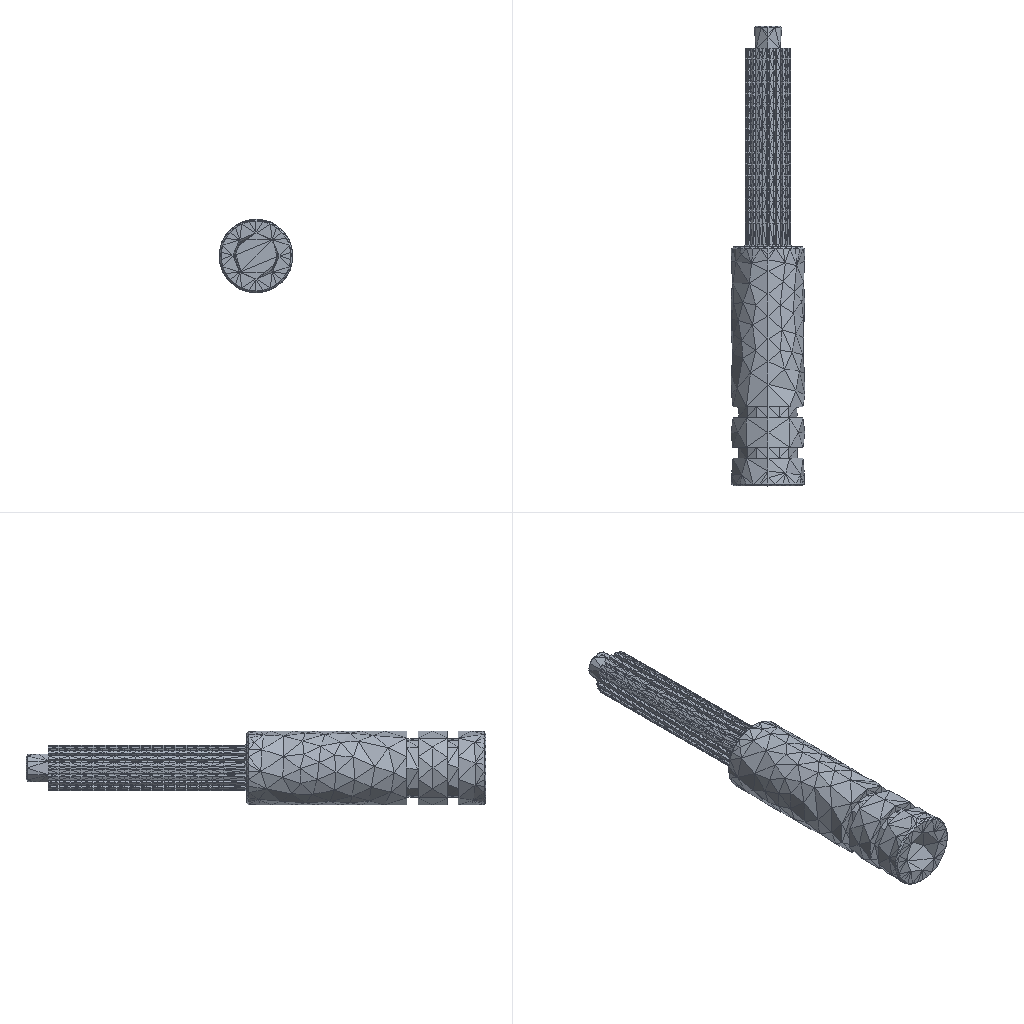Simulation study | ansys workbench
Ansys APDL input file, long lists of numbers shortened:
/batch
/config,noeldb,1     ! force off writing results to database
*get,_wallstrt,active,,time,wall
! ANSYS input file written by Workbench version 2022 R1
! File used for geometry attach: F:\ansys（分析文件汇总)\ansys转向器有限元分析\转向器\分析\齿条.STEP
/title,wbnew--____ (E5)
! ****** Begin Custom Load Command Snippet ******
/COM, ACT Extensions:
/COM,     LSDYNA, 2021.1
/COM,
! ****** End   Custom Load Command Snippet ******
*DIM,_wb_ProjectScratch_dir,string,248
_wb_ProjectScratch_dir(1) = 'C:\Users\Administrator\AppData\Local\Temp\WB_Administrator_18756_2\_ProjectScratch\Scr7D70\'
*DIM,_wb_SolverFiles_dir,string,248
_wb_SolverFiles_dir(1) = 'C:\Users\Administrator\AppData\Local\Temp\WB_Administrator_18756_2\wbnew_files\dp0\SYS-1\MECH\'
*DIM,_wb_userfiles_dir,string,248
_wb_userfiles_dir(1) = 'C:\Users\Administrator\AppData\Local\Temp\WB_Administrator_18756_2\wbnew_files\user_files\'
/com,--- Data in consistent NMM units. See Solving Units in the help system for more information.
/units,MPA
/nopr
/wb,file,start              !  signify a WB generated input file
/prep7
! Turn off shape checking because checks already performed inside WB mesher.
! See help system for more information.
SHPP,OFF,,NOWARN
/nolist
etcon,set             ! allow ANSYS to choose best KEYOP's for 180x elements, resets any applicable keyopt to MAPDL defaults
/com,*********** Nodes for the whole assembly ***********
nblock,3,,8393
(1i9,3e20.9e3)
        1    -9.866055935E-15    -3.500000000E+01     4.985000000E+02
! (7629 more lines like these left out)
-1
/wb,elem,start            !  set before creation of elements
/com,*********** Elements for Body 1 "__-FreeParts|__-__4" ***********
et,1,187
eblock,19,solid,,3600
(19i9)
        1        1        1        1        0        0        0        0       10        0        1      682     1334     1374     1348     5617     7596     5619     5618
! (7199 more lines like these left out)
-1
/wb,elem,end               !  done creating elements
/com,*********** Send User Defined Coordinate System(s) ***********
csys,0
toffst,273.15,  ! Temperature offset from absolute zero
/com,*********** Set Reference Temperature ***********
tref,22.
/wb,mat,start              !  starting to send materials
/com,*********** Send Materials ***********
Temperature = 'TEMP' ! Temperature
MP,DENS,1,7.85e-09,	! tonne mm^-3
MP,ALPX,1,1.2e-05,	! C^-1
MP,C,1,434000000,	! mm^2 s^-2 C^-1
MP,KXX,1,60.5,	! tonne mm s^-3 C^-1
MP,RSVX,1,0.00017,	! ohm mm
MP,EX,1,200000,	! tonne s^-2 mm^-1
MP,NUXY,1,0.3,
MP,MURX,1,10000,
/wb,mat,end                !  done sending materials
!************************* Model Summary ********************
!__-FreeParts|__-__4,	结构钢,	matid,	1
!************************* End Model Summary ********************
! get the diagonal of the bounding box. Needed later for other things
*get,_xmin,node,,mnloc,x
*get,_ymin,node,,mnloc,y
*get,_zmin,node,,mnloc,z
*get,_xmax,node,,mxloc,x
*get,_ymax,node,,mxloc,y
*get,_zmax,node,,mxloc,z
_ASMDIAG=(_xmax-_xmin)*(_xmax-_xmin)+(_ymax-_ymin)*(_ymax-_ymin)+(_zmax-_zmin)*(_zmax-_zmin)
_ASMDIAG=SQRT(_ASMDIAG)
/wb,contact,start          !  starting to send contact
/wb,contact,end            !  done creating contacts
/com,*********** Send Named Selection as Node Component ***********
CMBLOCK,______  ,NODE,      744
(8i10)
       207       208       211       212       215       216       219       220
! (92 more lines like these left out)
/golist
/wb,load,start             !  starting to send loads
/com,*********** Fixed Supports ***********
CMBLOCK,_FIXEDSU,NODE,      343
(8i10)
        21        22        23        24        25        36        37        38
! (42 more lines like these left out)
cmsel,s,_FIXEDSU
d,all,all
nsel,all
/com,*********** Define Force Using Surface Effect Elements ***********
local,12,0,0.,0.,0.,0.,0.,0.
csys,0
et,2,154
eblock,10,,,198
(15i9)
     6139        2        2        2       12      413      450      942      942     4067     4272      942     4072
! (197 more lines like these left out)
-1
esel,s,type,,2
keyop,2,2,1                ! Apply load in local coordinate system
keyop,2,7,1                ! Use original area so load is constant in large deformation
esel,all
/gst,on,on
fini
*get,_numnode,node,0,count
*get,_numelem,elem,0,count
*get, _MAXELEMNUM, elem, 0, NUM, MAX
*get, _MAXNODENUM, node, 0, NUM, MAX
*get, _MAXELEMTYPE, etyp, 0, NUM, MAX
*get, _MAXREALCONST, real, 0, NUM, MAX
/go
/wb,load,end               !  done creating loads
/com,--- Number of total nodes = %_numnode%
/com,--- Number of contact elements = 198
/com,--- Number of spring elements = 0
/com,--- Number of bearing elements = 0
/com,--- Number of solid elements = 3600
/com,--- Number of condensed parts = 0
/com,--- Number of total elements = %_numelem%
*get,_wallbsol,active,,time,wall
/com,****************************************************************************
/com,*************************    SOLUTION       ********************************
/com,****************************************************************************
/solu
antype,0                   ! static analysis
_thickRatio=  0     ! Ratio of thick parts in the model
eqsl,sparse,,,,,1
cntr,print,1               ! print out contact info and also make no initial contact an error
dmpoption,emat,no             ! Don't combine emat file for DANSYS
dmpoption,esav,no             ! Don't combine esav file for DANSYS
nldiag,cont,iter           ! print out contact info each equilibrium iteration
rescontrol,,none                 ! Do not keep any restart files
/com,****************************************************
/com,******************* SOLVE FOR LS 1 OF 1 ****************
esel,s,type,,2
nsle
sfe,all,1,pres,1,0.
sfe,all,2,pres,1,-3.35634495697455e-015
sfe,all,3,pres,1,1.818
nsel,all
esel,all
/nopr
/gopr
nsub,1,1,1
time,1.
outres,erase
outres,all,none
outres,nsol,all,
outres,rsol,all
outres,eangl,all
outres,etmp,all
outres,veng,all
outres,strs,all,
outres,epel,all,
outres,eppl,all,
outres,cont,all,
! *********** WB SOLVE COMMAND ***********
! check interactive state
*get,ANSINTER_,active,,int
*if,ANSINTER_,ne,0,then
/eof
*endif
solve
/com *************** Write FE CONNECTORS *********
CEWRITE,file,ce,,INTE
/com,****************************************************
/com,*************** FINISHED SOLVE FOR LS 1 *************
*get,_wallasol,active,,time,wall
/nopr
*get,_numnode,node,0,count
*get,_numelem,elem,0,count
*get, _MAXELEMNUM, elem, 0, NUM, MAX
*get, _MAXNODENUM, node, 0, NUM, MAX,,,INTERNAL
*get, _MAXELEMTYPE, etyp, 0, NUM, MAX
*get, _MAXREALCONST, real, 0, NUM, MAX
/gopr
/post1
xmlo,ENCODING,ISO-8859-1
xmlo,parm
/xml,parm,xml
fini
/gopr
*get,_walldone,active,,time,wall
_preptime=(_wallbsol-_wallstrt)*3600
_solvtime=(_wallasol-_wallbsol)*3600
_posttime=(_walldone-_wallasol)*3600
_totaltim=(_walldone-_wallstrt)*3600
*get,_dlbratio,active,0,solu,dlbr
*get,_combtime,active,0,solu,comb
*get,_ssmode,active,0,solu,ssmm
*get,_ndofs,active,0,solu,ndof
*get,_sol_end_time,active,0,set,time
*if,_sol_end_time,eq,1.,then
/fclean				!clean distributed files
*endif
/com,--- Total number of nodes = %_numnode%
/com,--- Total number of elements = %_numelem%
/com,--- Element load balance ratio = %_dlbratio%
/com,--- Time to combine distributed files = %_combtime%
/com,--- Sparse memory mode = %_ssmode%
/com,--- Number of DOF = %_ndofs%
/wb,file,end               ! done with WB generated input